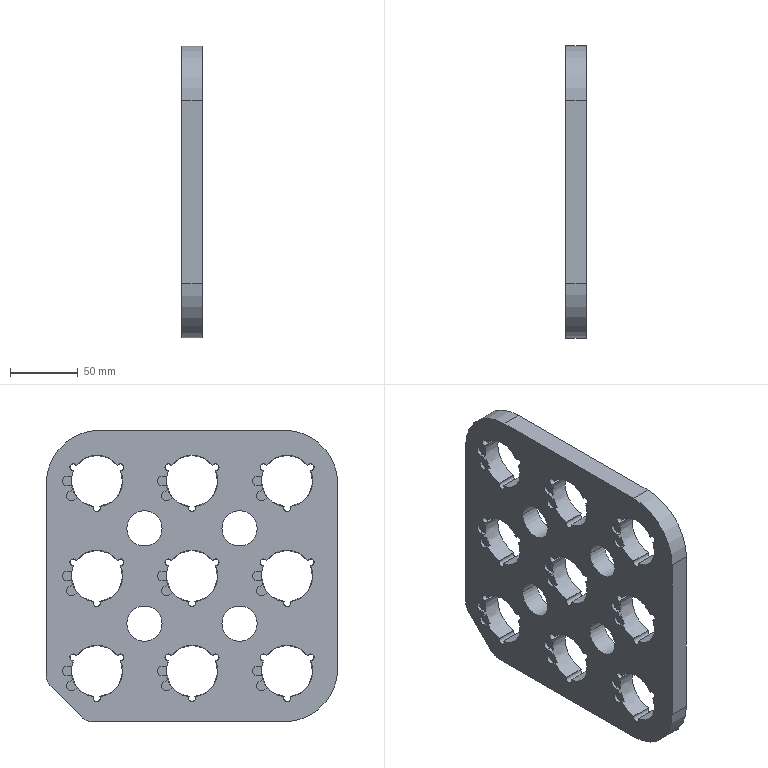Part | SolidWorks | features ICE 5, HoleWzd 3, Cut 2, Fillet 2, LPattern 2, Chamfer 1, Extrusion 1, RefAxis 1, RevCut 1 | 1 solid | 164 faces | box 15 x 215 x 215 mm | volume 479091 mm3 | cone 72 | plane 61 | cylinder 31 | commonest cylinder face diameters 7 x18 26 x8 80 x3 20 x2